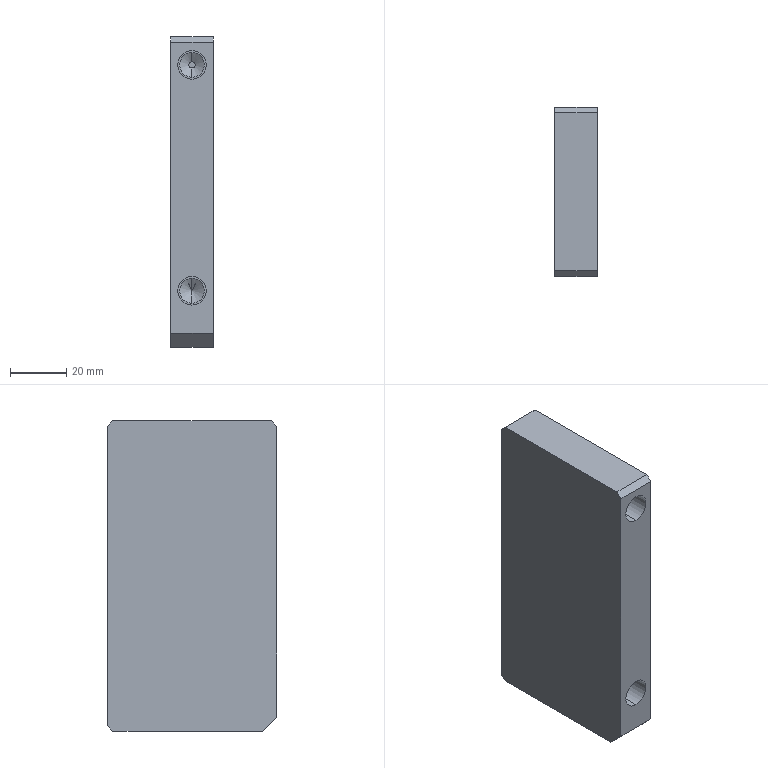Part | SolidWorks | features BaseBody 1 | 1 solid | 25 faces | box 15 x 60 x 110 mm | volume 93077 mm3 | plane 13 | cylinder 8 | cone 4 | commonest cylinder face diameters 8.8 x4 10.1 x4
STEP:
#1=CARTESIAN_POINT('',(257.5,55.,208.171));
#2=VERTEX_POINT('',#1);
#3=CARTESIAN_POINT('',(257.5,55.,198.071));
#4=VERTEX_POINT('',#3);
#5=CARTESIAN_POINT('',(257.5,55.,203.121));
#6=DIRECTION('',(0.,-1.,0.));
#7=DIRECTION('',(0.,0.,-1.));
#8=AXIS2_PLACEMENT_3D('',#5,#6,#7);
#9=CIRCLE('',#8,5.05);
#10=EDGE_CURVE('',#2,#4,#9,.T.);
#11=ORIENTED_EDGE('',*,*,#10,.F.);
#12=CARTESIAN_POINT('',(257.5,47.,208.171));
#13=VERTEX_POINT('',#12);
#14=CARTESIAN_POINT('',(257.5,55.,208.171));
#15=DIRECTION('',(0.,-1.,0.));
#16=VECTOR('',#15,1000.);
#17=LINE('',#14,#16);
#18=EDGE_CURVE('',#2,#13,#17,.T.);
#19=ORIENTED_EDGE('',*,*,#18,.T.);
#20=CARTESIAN_POINT('',(257.5,47.,198.071));
#21=VERTEX_POINT('',#20);
#22=CARTESIAN_POINT('',(257.5,47.,203.121));
#23=DIRECTION('',(0.,-1.,0.));
#24=DIRECTION('',(0.,0.,-1.));
#25=AXIS2_PLACEMENT_3D('',#22,#23,#24);
#26=CIRCLE('',#25,5.05);
#27=EDGE_CURVE('',#13,#21,#26,.T.);
#28=ORIENTED_EDGE('',*,*,#27,.T.);
#29=CARTESIAN_POINT('',(257.5,55.,198.071));
#30=DIRECTION('',(0.,-1.,0.));
#31=VECTOR('',#30,1000.);
#32=LINE('',#29,#31);
#33=EDGE_CURVE('',#4,#21,#32,.T.);
#34=ORIENTED_EDGE('',*,*,#33,.F.);
#35=EDGE_LOOP('',(#11,#19,#28,#34));
#36=FACE_OUTER_BOUND('',#35,.T.);
#37=CARTESIAN_POINT('',(257.5,55.,203.121));
#38=DIRECTION('',(0.,-1.,0.));
#39=DIRECTION('',(0.,0.,-1.));
#40=AXIS2_PLACEMENT_3D('',#37,#38,#39);
#41=CYLINDRICAL_SURFACE('',#40,5.05);
#42=ADVANCED_FACE('',(#36),#41,.F.);
#43=CARTESIAN_POINT('',(257.5,55.,128.171));
#44=VERTEX_POINT('',#43);
#45=CARTESIAN_POINT('',(257.5,55.,118.071));
#46=VERTEX_POINT('',#45);
#47=CARTESIAN_POINT('',(257.5,55.,123.121));
#48=DIRECTION('',(0.,-1.,0.));
#49=DIRECTION('',(0.,0.,-1.));
#50=AXIS2_PLACEMENT_3D('',#47,#48,#49);
#51=CIRCLE('',#50,5.05);
#52=EDGE_CURVE('',#44,#46,#51,.T.);
#53=ORIENTED_EDGE('',*,*,#52,.F.);
#54=CARTESIAN_POINT('',(257.5,47.,128.171));
#55=VERTEX_POINT('',#54);
#56=CARTESIAN_POINT('',(257.5,55.,128.171));
#57=DIRECTION('',(0.,-1.,0.));
#58=VECTOR('',#57,1000.);
#59=LINE('',#56,#58);
#60=EDGE_CURVE('',#44,#55,#59,.T.);
#61=ORIENTED_EDGE('',*,*,#60,.T.);
#62=CARTESIAN_POINT('',(257.5,47.,118.071));
#63=VERTEX_POINT('',#62);
#64=CARTESIAN_POINT('',(257.5,47.,123.121));
#65=DIRECTION('',(0.,-1.,0.));
#66=DIRECTION('',(0.,0.,-1.));
#67=AXIS2_PLACEMENT_3D('',#64,#65,#66);
#68=CIRCLE('',#67,5.05);
#69=EDGE_CURVE('',#55,#63,#68,.T.);
#70=ORIENTED_EDGE('',*,*,#69,.T.);
#71=CARTESIAN_POINT('',(257.5,55.,118.071));
#72=DIRECTION('',(0.,-1.,0.));
#73=VECTOR('',#72,1000.);
#74=LINE('',#71,#73);
#75=EDGE_CURVE('',#46,#63,#74,.T.);
#76=ORIENTED_EDGE('',*,*,#75,.F.);
#77=EDGE_LOOP('',(#53,#61,#70,#76));
#78=FACE_OUTER_BOUND('',#77,.T.);
#79=CARTESIAN_POINT('',(257.5,55.,123.121));
#80=DIRECTION('',(0.,-1.,0.));
#81=DIRECTION('',(0.,0.,-1.));
#82=AXIS2_PLACEMENT_3D('',#79,#80,#81);
#83=CYLINDRICAL_SURFACE('',#82,5.05);
#84=ADVANCED_FACE('',(#78),#83,.F.);
#85=CARTESIAN_POINT('',(257.5,90.,207.521));
#86=VERTEX_POINT('',#85);
#87=CARTESIAN_POINT('',(257.5,90.,198.721));
#88=VERTEX_POINT('',#87);
#89=CARTESIAN_POINT('',(257.5,90.,203.121));
#90=DIRECTION('',(0.,-1.,0.));
#91=DIRECTION('',(0.,0.,-1.));
#92=AXIS2_PLACEMENT_3D('',#89,#90,#91);
#93=CIRCLE('',#92,4.4);
#94=EDGE_CURVE('',#86,#88,#93,.T.);
#95=ORIENTED_EDGE('',*,*,#94,.F.);
#96=CARTESIAN_POINT('',(257.5,55.,207.521));
#97=VERTEX_POINT('',#96);
#98=CARTESIAN_POINT('',(257.5,55.,207.521));
#99=DIRECTION('',(0.,-1.,0.));
#100=VECTOR('',#99,1000.);
#101=LINE('',#98,#100);
#102=EDGE_CURVE('',#86,#97,#101,.T.);
#103=ORIENTED_EDGE('',*,*,#102,.T.);
#104=CARTESIAN_POINT('',(257.5,55.,198.721));
#105=VERTEX_POINT('',#104);
#106=CARTESIAN_POINT('',(257.5,55.,203.121));
#107=DIRECTION('',(0.,1.,0.));
#108=DIRECTION('',(0.,0.,-1.));
#109=AXIS2_PLACEMENT_3D('',#106,#107,#108);
#110=CIRCLE('',#109,4.4);
#111=EDGE_CURVE('',#105,#97,#110,.T.);
#112=ORIENTED_EDGE('',*,*,#111,.F.);
#113=CARTESIAN_POINT('',(257.5,55.,198.721));
#114=DIRECTION('',(0.,-1.,0.));
#115=VECTOR('',#114,1000.);
#116=LINE('',#113,#115);
#117=EDGE_CURVE('',#88,#105,#116,.T.);
#118=ORIENTED_EDGE('',*,*,#117,.F.);
#119=EDGE_LOOP('',(#95,#103,#112,#118));
#120=FACE_OUTER_BOUND('',#119,.T.);
#121=CARTESIAN_POINT('',(257.5,55.,203.121));
#122=DIRECTION('',(0.,-1.,0.));
#123=DIRECTION('',(0.,0.,-1.));
#124=AXIS2_PLACEMENT_3D('',#121,#122,#123);
#125=CYLINDRICAL_SURFACE('',#124,4.4);
#126=ADVANCED_FACE('',(#120),#125,.F.);
#127=CARTESIAN_POINT('',(257.5,90.,127.521));
#128=VERTEX_POINT('',#127);
#129=CARTESIAN_POINT('',(257.5,90.,118.721));
#130=VERTEX_POINT('',#129);
#131=CARTESIAN_POINT('',(257.5,90.,123.121));
#132=DIRECTION('',(0.,-1.,0.));
#133=DIRECTION('',(0.,0.,-1.));
#134=AXIS2_PLACEMENT_3D('',#131,#132,#133);
#135=CIRCLE('',#134,4.4);
#136=EDGE_CURVE('',#128,#130,#135,.T.);
#137=ORIENTED_EDGE('',*,*,#136,.F.);
#138=CARTESIAN_POINT('',(257.5,55.,127.521));
#139=VERTEX_POINT('',#138);
#140=CARTESIAN_POINT('',(257.5,55.,127.521));
#141=DIRECTION('',(0.,-1.,0.));
#142=VECTOR('',#141,1000.);
#143=LINE('',#140,#142);
#144=EDGE_CURVE('',#128,#139,#143,.T.);
#145=ORIENTED_EDGE('',*,*,#144,.T.);
#146=CARTESIAN_POINT('',(257.5,55.,118.721));
#147=VERTEX_POINT('',#146);
#148=CARTESIAN_POINT('',(257.5,55.,123.121));
#149=DIRECTION('',(0.,1.,0.));
#150=DIRECTION('',(0.,0.,-1.));
#151=AXIS2_PLACEMENT_3D('',#148,#149,#150);
#152=CIRCLE('',#151,4.4);
#153=EDGE_CURVE('',#147,#139,#152,.T.);
#154=ORIENTED_EDGE('',*,*,#153,.F.);
#155=CARTESIAN_POINT('',(257.5,55.,118.721));
#156=DIRECTION('',(0.,-1.,0.));
#157=VECTOR('',#156,1000.);
#158=LINE('',#155,#157);
#159=EDGE_CURVE('',#130,#147,#158,.T.);
#160=ORIENTED_EDGE('',*,*,#159,.F.);
#161=EDGE_LOOP('',(#137,#145,#154,#160));
#162=FACE_OUTER_BOUND('',#161,.T.);
#163=CARTESIAN_POINT('',(257.5,55.,123.121));
#164=DIRECTION('',(0.,-1.,0.));
#165=DIRECTION('',(0.,0.,-1.));
#166=AXIS2_PLACEMENT_3D('',#163,#164,#165);
#167=CYLINDRICAL_SURFACE('',#166,4.4);
#168=ADVANCED_FACE('',(#162),#167,.F.);
#169=CARTESIAN_POINT('',(257.5,92.,204.193));
#170=VERTEX_POINT('',#169);
#171=CARTESIAN_POINT('',(257.5,92.,202.05));
#172=VERTEX_POINT('',#171);
#173=CARTESIAN_POINT('',(257.5,92.,203.121));
#174=DIRECTION('',(0.,-1.,0.));
#175=DIRECTION('',(0.,0.,-1.));
#176=AXIS2_PLACEMENT_3D('',#173,#174,#175);
#177=CIRCLE('',#176,1.071);
#178=EDGE_CURVE('',#170,#172,#177,.T.);
#179=ORIENTED_EDGE('',*,*,#178,.F.);
#180=CARTESIAN_POINT('',(257.5,90.,207.521));
#181=DIRECTION('',(0.,-0.515,0.8572));
#182=VECTOR('',#181,1000.);
#183=LINE('',#180,#182);
#184=EDGE_CURVE('',#170,#86,#183,.T.);
#185=ORIENTED_EDGE('',*,*,#184,.T.);
#186=ORIENTED_EDGE('',*,*,#94,.T.);
#187=CARTESIAN_POINT('',(257.5,90.,198.721));
#188=DIRECTION('',(0.,-0.515,-0.8572));
#189=VECTOR('',#188,1000.);
#190=LINE('',#187,#189);
#191=EDGE_CURVE('',#172,#88,#190,.T.);
#192=ORIENTED_EDGE('',*,*,#191,.F.);
#193=EDGE_LOOP('',(#179,#185,#186,#192));
#194=FACE_OUTER_BOUND('',#193,.T.);
#195=CARTESIAN_POINT('',(257.5,90.,203.121));
#196=DIRECTION('',(0.,-1.,0.));
#197=DIRECTION('',(0.,0.,-1.));
#198=AXIS2_PLACEMENT_3D('',#195,#196,#197);
#199=CONICAL_SURFACE('',#198,4.4,1.03);
#200=ADVANCED_FACE('',(#194),#199,.F.);
#201=CARTESIAN_POINT('',(257.5,92.644,123.121));
#202=VERTEX_POINT('',#201);
#203=CARTESIAN_POINT('',(257.5,90.,118.721));
#204=DIRECTION('',(0.,-0.515,-0.8572));
#205=VECTOR('',#204,1000.);
#206=LINE('',#203,#205);
#207=EDGE_CURVE('',#202,#130,#206,.T.);
#208=ORIENTED_EDGE('',*,*,#207,.F.);
#209=CARTESIAN_POINT('',(257.5,90.,127.521));
#210=DIRECTION('',(0.,-0.515,0.8572));
#211=VECTOR('',#210,1000.);
#212=LINE('',#209,#211);
#213=EDGE_CURVE('',#202,#128,#212,.T.);
#214=ORIENTED_EDGE('',*,*,#213,.T.);
#215=ORIENTED_EDGE('',*,*,#136,.T.);
#216=EDGE_LOOP('',(#208,#214,#215));
#217=FACE_OUTER_BOUND('',#216,.T.);
#218=CARTESIAN_POINT('',(257.5,90.,123.121));
#219=DIRECTION('',(0.,-1.,0.));
#220=DIRECTION('',(0.,0.,-1.));
#221=AXIS2_PLACEMENT_3D('',#218,#219,#220);
#222=CONICAL_SURFACE('',#221,4.4,1.03);
#223=ADVANCED_FACE('',(#217),#222,.F.);
#224=CARTESIAN_POINT('',(250.,105.,103.121));
#225=VERTEX_POINT('',#224);
#226=CARTESIAN_POINT('',(250.,107.,105.121));
#227=VERTEX_POINT('',#226);
#228=CARTESIAN_POINT('',(250.,105.,103.121));
#229=DIRECTION('',(0.,0.7071,0.7071));
#230=VECTOR('',#229,1000.);
#231=LINE('',#228,#230);
#232=EDGE_CURVE('',#225,#227,#231,.T.);
#233=ORIENTED_EDGE('',*,*,#232,.F.);
#234=CARTESIAN_POINT('',(250.,52.,103.121));
#235=VERTEX_POINT('',#234);
#236=CARTESIAN_POINT('',(250.,47.,103.121));
#237=DIRECTION('',(0.,1.,0.));
#238=VECTOR('',#237,1000.);
#239=LINE('',#236,#238);
#240=EDGE_CURVE('',#235,#225,#239,.T.);
#241=ORIENTED_EDGE('',*,*,#240,.F.);
#242=CARTESIAN_POINT('',(250.,47.,108.121));
#243=VERTEX_POINT('',#242);
#244=CARTESIAN_POINT('',(250.,47.,108.121));
#245=DIRECTION('',(0.,0.7071,-0.7071));
#246=VECTOR('',#245,1000.);
#247=LINE('',#244,#246);
#248=EDGE_CURVE('',#243,#235,#247,.T.);
#249=ORIENTED_EDGE('',*,*,#248,.F.);
#250=CARTESIAN_POINT('',(250.,47.,211.121));
#251=VERTEX_POINT('',#250);
#252=CARTESIAN_POINT('',(250.,47.,103.121));
#253=DIRECTION('',(0.,0.,-1.));
#254=VECTOR('',#253,1000.);
#255=LINE('',#252,#254);
#256=EDGE_CURVE('',#251,#243,#255,.T.);
#257=ORIENTED_EDGE('',*,*,#256,.F.);
#258=CARTESIAN_POINT('',(250.,49.,213.121));
#259=VERTEX_POINT('',#258);
#260=CARTESIAN_POINT('',(250.,49.,213.121));
#261=DIRECTION('',(0.,-0.7071,-0.7071));
#262=VECTOR('',#261,1000.);
#263=LINE('',#260,#262);
#264=EDGE_CURVE('',#259,#251,#263,.T.);
#265=ORIENTED_EDGE('',*,*,#264,.F.);
#266=CARTESIAN_POINT('',(250.,105.,213.121));
#267=VERTEX_POINT('',#266);
#268=CARTESIAN_POINT('',(250.,47.,213.121));
#269=DIRECTION('',(0.,-1.,0.));
#270=VECTOR('',#269,1000.);
#271=LINE('',#268,#270);
#272=EDGE_CURVE('',#267,#259,#271,.T.);
#273=ORIENTED_EDGE('',*,*,#272,.F.);
#274=CARTESIAN_POINT('',(250.,107.,211.121));
#275=VERTEX_POINT('',#274);
#276=CARTESIAN_POINT('',(250.,107.,211.121));
#277=DIRECTION('',(0.,-0.7071,0.7071));
#278=VECTOR('',#277,1000.);
#279=LINE('',#276,#278);
#280=EDGE_CURVE('',#275,#267,#279,.T.);
#281=ORIENTED_EDGE('',*,*,#280,.F.);
#282=CARTESIAN_POINT('',(250.,107.,103.121));
#283=DIRECTION('',(0.,0.,1.));
#284=VECTOR('',#283,1000.);
#285=LINE('',#282,#284);
#286=EDGE_CURVE('',#227,#275,#285,.T.);
#287=ORIENTED_EDGE('',*,*,#286,.F.);
#288=EDGE_LOOP('',(#233,#241,#249,#257,#265,#273,#281,#287));
#289=FACE_OUTER_BOUND('',#288,.T.);
#290=CARTESIAN_POINT('',(250.,47.,103.121));
#291=DIRECTION('',(1.,0.,0.));
#292=DIRECTION('',(0.,0.,-1.));
#293=AXIS2_PLACEMENT_3D('',#290,#291,#292);
#294=PLANE('',#293);
#295=ADVANCED_FACE('',(#289),#294,.F.);
#296=CARTESIAN_POINT('',(265.,107.,105.121));
#297=VERTEX_POINT('',#296);
#298=CARTESIAN_POINT('',(177.5,107.,105.121));
#299=DIRECTION('',(1.,0.,0.));
#300=VECTOR('',#299,1000.);
#301=LINE('',#298,#300);
#302=EDGE_CURVE('',#227,#297,#301,.T.);
#303=ORIENTED_EDGE('',*,*,#302,.F.);
#304=ORIENTED_EDGE('',*,*,#286,.T.);
#305=CARTESIAN_POINT('',(265.,107.,211.121));
#306=VERTEX_POINT('',#305);
#307=CARTESIAN_POINT('',(177.5,107.,211.121));
#308=DIRECTION('',(-1.,0.,0.));
#309=VECTOR('',#308,1000.);
#310=LINE('',#307,#309);
#311=EDGE_CURVE('',#306,#275,#310,.T.);
#312=ORIENTED_EDGE('',*,*,#311,.F.);
#313=CARTESIAN_POINT('',(265.,107.,153.121));
#314=DIRECTION('',(0.,0.,1.));
#315=VECTOR('',#314,1000.);
#316=LINE('',#313,#315);
#317=EDGE_CURVE('',#297,#306,#316,.T.);
#318=ORIENTED_EDGE('',*,*,#317,.F.);
#319=EDGE_LOOP('',(#303,#304,#312,#318));
#320=FACE_OUTER_BOUND('',#319,.T.);
#321=CARTESIAN_POINT('',(177.5,107.,153.121));
#322=DIRECTION('',(0.,-1.,0.));
#323=DIRECTION('',(0.,0.,-1.));
#324=AXIS2_PLACEMENT_3D('',#321,#322,#323);
#325=PLANE('',#324);
#326=ADVANCED_FACE('',(#320),#325,.F.);
#327=ORIENTED_EDGE('',*,*,#302,.T.);
#328=CARTESIAN_POINT('',(265.,105.,103.121));
#329=VERTEX_POINT('',#328);
#330=CARTESIAN_POINT('',(265.,105.,103.121));
#331=DIRECTION('',(0.,0.7071,0.7071));
#332=VECTOR('',#331,1000.);
#333=LINE('',#330,#332);
#334=EDGE_CURVE('',#329,#297,#333,.T.);
#335=ORIENTED_EDGE('',*,*,#334,.F.);
#336=CARTESIAN_POINT('',(90.,105.,103.121));
#337=DIRECTION('',(1.,0.,0.));
#338=VECTOR('',#337,1000.);
#339=LINE('',#336,#338);
#340=EDGE_CURVE('',#225,#329,#339,.T.);
#341=ORIENTED_EDGE('',*,*,#340,.F.);
#342=ORIENTED_EDGE('',*,*,#232,.T.);
#343=EDGE_LOOP('',(#327,#335,#341,#342));
#344=FACE_OUTER_BOUND('',#343,.T.);
#345=CARTESIAN_POINT('',(90.,105.,103.121));
#346=DIRECTION('',(0.,-0.7071,0.7071));
#347=DIRECTION('',(0.,-0.7071,-0.7071));
#348=AXIS2_PLACEMENT_3D('',#345,#346,#347);
#349=PLANE('',#348);
#350=ADVANCED_FACE('',(#344),#349,.F.);
#351=ORIENTED_EDGE('',*,*,#340,.T.);
#352=CARTESIAN_POINT('',(265.,52.,103.121));
#353=VERTEX_POINT('',#352);
#354=CARTESIAN_POINT('',(265.,92.,103.121));
#355=DIRECTION('',(0.,1.,0.));
#356=VECTOR('',#355,1000.);
#357=LINE('',#354,#356);
#358=EDGE_CURVE('',#353,#329,#357,.T.);
#359=ORIENTED_EDGE('',*,*,#358,.F.);
#360=CARTESIAN_POINT('',(90.,52.,103.121));
#361=DIRECTION('',(1.,0.,0.));
#362=VECTOR('',#361,1000.);
#363=LINE('',#360,#362);
#364=EDGE_CURVE('',#235,#353,#363,.T.);
#365=ORIENTED_EDGE('',*,*,#364,.F.);
#366=ORIENTED_EDGE('',*,*,#240,.T.);
#367=EDGE_LOOP('',(#351,#359,#365,#366));
#368=FACE_OUTER_BOUND('',#367,.T.);
#369=CARTESIAN_POINT('',(90.,92.,103.121));
#370=DIRECTION('',(0.,0.,1.));
#371=DIRECTION('',(1.,0.,0.));
#372=AXIS2_PLACEMENT_3D('',#369,#370,#371);
#373=PLANE('',#372);
#374=ADVANCED_FACE('',(#368),#373,.F.);
#375=ORIENTED_EDGE('',*,*,#364,.T.);
#376=CARTESIAN_POINT('',(265.,47.,108.121));
#377=VERTEX_POINT('',#376);
#378=CARTESIAN_POINT('',(265.,47.,108.121));
#379=DIRECTION('',(0.,0.7071,-0.7071));
#380=VECTOR('',#379,1000.);
#381=LINE('',#378,#380);
#382=EDGE_CURVE('',#377,#353,#381,.T.);
#383=ORIENTED_EDGE('',*,*,#382,.F.);
#384=CARTESIAN_POINT('',(177.5,47.,108.121));
#385=DIRECTION('',(1.,0.,0.));
#386=VECTOR('',#385,1000.);
#387=LINE('',#384,#386);
#388=EDGE_CURVE('',#243,#377,#387,.T.);
#389=ORIENTED_EDGE('',*,*,#388,.F.);
#390=ORIENTED_EDGE('',*,*,#248,.T.);
#391=EDGE_LOOP('',(#375,#383,#389,#390));
#392=FACE_OUTER_BOUND('',#391,.T.);
#393=CARTESIAN_POINT('',(177.5,47.,108.121));
#394=DIRECTION('',(0.,0.7071,0.7071));
#395=DIRECTION('',(0.,-0.7071,0.7071));
#396=AXIS2_PLACEMENT_3D('',#393,#394,#395);
#397=PLANE('',#396);
#398=ADVANCED_FACE('',(#392),#397,.F.);
#399=CARTESIAN_POINT('',(265.,47.,211.121));
#400=VERTEX_POINT('',#399);
#401=CARTESIAN_POINT('',(177.5,47.,211.121));
#402=DIRECTION('',(1.,0.,0.));
#403=VECTOR('',#402,1000.);
#404=LINE('',#401,#403);
#405=EDGE_CURVE('',#251,#400,#404,.T.);
#406=ORIENTED_EDGE('',*,*,#405,.F.);
#407=ORIENTED_EDGE('',*,*,#256,.T.);
#408=ORIENTED_EDGE('',*,*,#388,.T.);
#409=CARTESIAN_POINT('',(265.,47.,153.121));
#410=DIRECTION('',(0.,0.,-1.));
#411=VECTOR('',#410,1000.);
#412=LINE('',#409,#411);
#413=EDGE_CURVE('',#400,#377,#412,.T.);
#414=ORIENTED_EDGE('',*,*,#413,.F.);
#415=EDGE_LOOP('',(#406,#407,#408,#414));
#416=FACE_OUTER_BOUND('',#415,.T.);
#417=CARTESIAN_POINT('',(257.5,47.,203.121));
#418=DIRECTION('',(0.,-1.,0.));
#419=DIRECTION('',(0.,0.,-1.));
#420=AXIS2_PLACEMENT_3D('',#417,#418,#419);
#421=CIRCLE('',#420,5.05);
#422=EDGE_CURVE('',#21,#13,#421,.T.);
#423=ORIENTED_EDGE('',*,*,#422,.F.);
#424=ORIENTED_EDGE('',*,*,#27,.F.);
#425=EDGE_LOOP('',(#423,#424));
#426=FACE_BOUND('',#425,.T.);
#427=CARTESIAN_POINT('',(257.5,47.,123.121));
#428=DIRECTION('',(0.,-1.,0.));
#429=DIRECTION('',(0.,0.,-1.));
#430=AXIS2_PLACEMENT_3D('',#427,#428,#429);
#431=CIRCLE('',#430,5.05);
#432=EDGE_CURVE('',#63,#55,#431,.T.);
#433=ORIENTED_EDGE('',*,*,#432,.F.);
#434=ORIENTED_EDGE('',*,*,#69,.F.);
#435=EDGE_LOOP('',(#433,#434));
#436=FACE_BOUND('',#435,.T.);
#437=CARTESIAN_POINT('',(177.5,47.,153.121));
#438=DIRECTION('',(0.,1.,0.));
#439=DIRECTION('',(0.,0.,1.));
#440=AXIS2_PLACEMENT_3D('',#437,#438,#439);
#441=PLANE('',#440);
#442=ADVANCED_FACE('',(#416,#426,#436),#441,.F.);
#443=CARTESIAN_POINT('',(265.,49.,213.121));
#444=VERTEX_POINT('',#443);
#445=CARTESIAN_POINT('',(265.,49.,213.121));
#446=DIRECTION('',(0.,0.7071,0.7071));
#447=VECTOR('',#446,1000.);
#448=LINE('',#445,#447);
#449=EDGE_CURVE('',#400,#444,#448,.T.);
#450=ORIENTED_EDGE('',*,*,#449,.T.);
#451=CARTESIAN_POINT('',(177.5,49.,213.121));
#452=DIRECTION('',(-1.,0.,0.));
#453=VECTOR('',#452,1000.);
#454=LINE('',#451,#453);
#455=EDGE_CURVE('',#444,#259,#454,.T.);
#456=ORIENTED_EDGE('',*,*,#455,.T.);
#457=ORIENTED_EDGE('',*,*,#264,.T.);
#458=ORIENTED_EDGE('',*,*,#405,.T.);
#459=EDGE_LOOP('',(#450,#456,#457,#458));
#460=FACE_OUTER_BOUND('',#459,.T.);
#461=CARTESIAN_POINT('',(177.5,49.,213.121));
#462=DIRECTION('',(0.,-0.7071,0.7071));
#463=DIRECTION('',(0.,-0.7071,-0.7071));
#464=AXIS2_PLACEMENT_3D('',#461,#462,#463);
#465=PLANE('',#464);
#466=ADVANCED_FACE('',(#460),#465,.T.);
#467=ORIENTED_EDGE('',*,*,#272,.T.);
#468=ORIENTED_EDGE('',*,*,#455,.F.);
#469=CARTESIAN_POINT('',(265.,105.,213.121));
#470=VERTEX_POINT('',#469);
#471=CARTESIAN_POINT('',(265.,107.,213.121));
#472=DIRECTION('',(0.,1.,0.));
#473=VECTOR('',#472,1000.);
#474=LINE('',#471,#473);
#475=EDGE_CURVE('',#444,#470,#474,.T.);
#476=ORIENTED_EDGE('',*,*,#475,.T.);
#477=CARTESIAN_POINT('',(177.5,105.,213.121));
#478=DIRECTION('',(-1.,0.,0.));
#479=VECTOR('',#478,1000.);
#480=LINE('',#477,#479);
#481=EDGE_CURVE('',#470,#267,#480,.T.);
#482=ORIENTED_EDGE('',*,*,#481,.T.);
#483=EDGE_LOOP('',(#467,#468,#476,#482));
#484=FACE_OUTER_BOUND('',#483,.T.);
#485=CARTESIAN_POINT('',(177.5,107.,213.121));
#486=DIRECTION('',(0.,0.,1.));
#487=DIRECTION('',(1.,0.,0.));
#488=AXIS2_PLACEMENT_3D('',#485,#486,#487);
#489=PLANE('',#488);
#490=ADVANCED_FACE('',(#484),#489,.T.);
#491=CARTESIAN_POINT('',(265.,107.,211.121));
#492=DIRECTION('',(0.,0.7071,-0.7071));
#493=VECTOR('',#492,1000.);
#494=LINE('',#491,#493);
#495=EDGE_CURVE('',#470,#306,#494,.T.);
#496=ORIENTED_EDGE('',*,*,#495,.T.);
#497=ORIENTED_EDGE('',*,*,#311,.T.);
#498=ORIENTED_EDGE('',*,*,#280,.T.);
#499=ORIENTED_EDGE('',*,*,#481,.F.);
#500=EDGE_LOOP('',(#496,#497,#498,#499));
#501=FACE_OUTER_BOUND('',#500,.T.);
#502=CARTESIAN_POINT('',(177.5,107.,211.121));
#503=DIRECTION('',(0.,0.7071,0.7071));
#504=DIRECTION('',(0.,-0.7071,0.7071));
#505=AXIS2_PLACEMENT_3D('',#502,#503,#504);
#506=PLANE('',#505);
#507=ADVANCED_FACE('',(#501),#506,.T.);
#508=ORIENTED_EDGE('',*,*,#334,.T.);
#509=ORIENTED_EDGE('',*,*,#317,.T.);
#510=ORIENTED_EDGE('',*,*,#495,.F.);
#511=ORIENTED_EDGE('',*,*,#475,.F.);
#512=ORIENTED_EDGE('',*,*,#449,.F.);
#513=ORIENTED_EDGE('',*,*,#413,.T.);
#514=ORIENTED_EDGE('',*,*,#382,.T.);
#515=ORIENTED_EDGE('',*,*,#358,.T.);
#516=EDGE_LOOP('',(#508,#509,#510,#511,#512,#513,#514,#515));
#517=FACE_OUTER_BOUND('',#516,.T.);
#518=CARTESIAN_POINT('',(265.,92.,103.121));
#519=DIRECTION('',(-1.,0.,0.));
#520=DIRECTION('',(0.,0.,1.));
#521=AXIS2_PLACEMENT_3D('',#518,#519,#520);
#522=PLANE('',#521);
#523=ADVANCED_FACE('',(#517),#522,.F.);
#524=ORIENTED_EDGE('',*,*,#18,.F.);
#525=CARTESIAN_POINT('',(257.5,55.,203.121));
#526=DIRECTION('',(0.,-1.,0.));
#527=DIRECTION('',(0.,0.,-1.));
#528=AXIS2_PLACEMENT_3D('',#525,#526,#527);
#529=CIRCLE('',#528,5.05);
#530=EDGE_CURVE('',#4,#2,#529,.T.);
#531=ORIENTED_EDGE('',*,*,#530,.F.);
#532=ORIENTED_EDGE('',*,*,#33,.T.);
#533=ORIENTED_EDGE('',*,*,#422,.T.);
#534=EDGE_LOOP('',(#524,#531,#532,#533));
#535=FACE_OUTER_BOUND('',#534,.T.);
#536=CARTESIAN_POINT('',(257.5,55.,203.121));
#537=DIRECTION('',(0.,-1.,0.));
#538=DIRECTION('',(0.,0.,-1.));
#539=AXIS2_PLACEMENT_3D('',#536,#537,#538);
#540=CYLINDRICAL_SURFACE('',#539,5.05);
#541=ADVANCED_FACE('',(#535),#540,.F.);
#542=ORIENTED_EDGE('',*,*,#60,.F.);
#543=CARTESIAN_POINT('',(257.5,55.,123.121));
#544=DIRECTION('',(0.,-1.,0.));
#545=DIRECTION('',(0.,0.,-1.));
#546=AXIS2_PLACEMENT_3D('',#543,#544,#545);
#547=CIRCLE('',#546,5.05);
#548=EDGE_CURVE('',#46,#44,#547,.T.);
#549=ORIENTED_EDGE('',*,*,#548,.F.);
#550=ORIENTED_EDGE('',*,*,#75,.T.);
#551=ORIENTED_EDGE('',*,*,#432,.T.);
#552=EDGE_LOOP('',(#542,#549,#550,#551));
#553=FACE_OUTER_BOUND('',#552,.T.);
#554=CARTESIAN_POINT('',(257.5,55.,123.121));
#555=DIRECTION('',(0.,-1.,0.));
#556=DIRECTION('',(0.,0.,-1.));
#557=AXIS2_PLACEMENT_3D('',#554,#555,#556);
#558=CYLINDRICAL_SURFACE('',#557,5.05);
#559=ADVANCED_FACE('',(#553),#558,.F.);
#560=ORIENTED_EDGE('',*,*,#530,.T.);
#561=ORIENTED_EDGE('',*,*,#10,.T.);
#562=EDGE_LOOP('',(#560,#561));
#563=FACE_OUTER_BOUND('',#562,.T.);
#564=ORIENTED_EDGE('',*,*,#111,.T.);
#565=CARTESIAN_POINT('',(257.5,55.,203.121));
#566=DIRECTION('',(0.,1.,0.));
#567=DIRECTION('',(0.,0.,-1.));
#568=AXIS2_PLACEMENT_3D('',#565,#566,#567);
#569=CIRCLE('',#568,4.4);
#570=EDGE_CURVE('',#97,#105,#569,.T.);
#571=ORIENTED_EDGE('',*,*,#570,.T.);
#572=EDGE_LOOP('',(#564,#571));
#573=FACE_BOUND('',#572,.T.);
#574=CARTESIAN_POINT('',(257.5,55.,203.121));
#575=DIRECTION('',(0.,-1.,0.));
#576=DIRECTION('',(0.,0.,-1.));
#577=AXIS2_PLACEMENT_3D('',#574,#575,#576);
#578=PLANE('',#577);
#579=ADVANCED_FACE('',(#563,#573),#578,.T.);
#580=ORIENTED_EDGE('',*,*,#548,.T.);
#581=ORIENTED_EDGE('',*,*,#52,.T.);
#582=EDGE_LOOP('',(#580,#581));
#583=FACE_OUTER_BOUND('',#582,.T.);
#584=ORIENTED_EDGE('',*,*,#153,.T.);
#585=CARTESIAN_POINT('',(257.5,55.,123.121));
#586=DIRECTION('',(0.,1.,0.));
#587=DIRECTION('',(0.,0.,-1.));
#588=AXIS2_PLACEMENT_3D('',#585,#586,#587);
#589=CIRCLE('',#588,4.4);
#590=EDGE_CURVE('',#139,#147,#589,.T.);
#591=ORIENTED_EDGE('',*,*,#590,.T.);
#592=EDGE_LOOP('',(#584,#591));
#593=FACE_BOUND('',#592,.T.);
#594=CARTESIAN_POINT('',(257.5,55.,123.121));
#595=DIRECTION('',(0.,-1.,0.));
#596=DIRECTION('',(0.,0.,-1.));
#597=AXIS2_PLACEMENT_3D('',#594,#595,#596);
#598=PLANE('',#597);
#599=ADVANCED_FACE('',(#583,#593),#598,.T.);
#600=ORIENTED_EDGE('',*,*,#102,.F.);
#601=CARTESIAN_POINT('',(257.5,90.,203.121));
#602=DIRECTION('',(0.,-1.,0.));
#603=DIRECTION('',(0.,0.,-1.));
#604=AXIS2_PLACEMENT_3D('',#601,#602,#603);
#605=CIRCLE('',#604,4.4);
#606=EDGE_CURVE('',#88,#86,#605,.T.);
#607=ORIENTED_EDGE('',*,*,#606,.F.);
#608=ORIENTED_EDGE('',*,*,#117,.T.);
#609=ORIENTED_EDGE('',*,*,#570,.F.);
#610=EDGE_LOOP('',(#600,#607,#608,#609));
#611=FACE_OUTER_BOUND('',#610,.T.);
#612=CARTESIAN_POINT('',(257.5,55.,203.121));
#613=DIRECTION('',(0.,-1.,0.));
#614=DIRECTION('',(0.,0.,-1.));
#615=AXIS2_PLACEMENT_3D('',#612,#613,#614);
#616=CYLINDRICAL_SURFACE('',#615,4.4);
#617=ADVANCED_FACE('',(#611),#616,.F.);
#618=ORIENTED_EDGE('',*,*,#144,.F.);
#619=CARTESIAN_POINT('',(257.5,90.,123.121));
#620=DIRECTION('',(0.,-1.,0.));
#621=DIRECTION('',(0.,0.,-1.));
#622=AXIS2_PLACEMENT_3D('',#619,#620,#621);
#623=CIRCLE('',#622,4.4);
#624=EDGE_CURVE('',#130,#128,#623,.T.);
#625=ORIENTED_EDGE('',*,*,#624,.F.);
#626=ORIENTED_EDGE('',*,*,#159,.T.);
#627=ORIENTED_EDGE('',*,*,#590,.F.);
#628=EDGE_LOOP('',(#618,#625,#626,#627));
#629=FACE_OUTER_BOUND('',#628,.T.);
#630=CARTESIAN_POINT('',(257.5,55.,123.121));
#631=DIRECTION('',(0.,-1.,0.));
#632=DIRECTION('',(0.,0.,-1.));
#633=AXIS2_PLACEMENT_3D('',#630,#631,#632);
#634=CYLINDRICAL_SURFACE('',#633,4.4);
#635=ADVANCED_FACE('',(#629),#634,.F.);
#636=ORIENTED_EDGE('',*,*,#184,.F.);
#637=CARTESIAN_POINT('',(257.5,92.,203.121));
#638=DIRECTION('',(0.,-1.,0.));
#639=DIRECTION('',(0.,0.,-1.));
#640=AXIS2_PLACEMENT_3D('',#637,#638,#639);
#641=CIRCLE('',#640,1.071);
#642=EDGE_CURVE('',#172,#170,#641,.T.);
#643=ORIENTED_EDGE('',*,*,#642,.F.);
#644=ORIENTED_EDGE('',*,*,#191,.T.);
#645=ORIENTED_EDGE('',*,*,#606,.T.);
#646=EDGE_LOOP('',(#636,#643,#644,#645));
#647=FACE_OUTER_BOUND('',#646,.T.);
#648=CARTESIAN_POINT('',(257.5,90.,203.121));
#649=DIRECTION('',(0.,-1.,0.));
#650=DIRECTION('',(0.,0.,-1.));
#651=AXIS2_PLACEMENT_3D('',#648,#649,#650);
#652=CONICAL_SURFACE('',#651,4.4,1.03);
#653=ADVANCED_FACE('',(#647),#652,.F.);
#654=ORIENTED_EDGE('',*,*,#213,.F.);
#655=ORIENTED_EDGE('',*,*,#207,.T.);
#656=ORIENTED_EDGE('',*,*,#624,.T.);
#657=EDGE_LOOP('',(#654,#655,#656));
#658=FACE_OUTER_BOUND('',#657,.T.);
#659=CARTESIAN_POINT('',(257.5,90.,123.121));
#660=DIRECTION('',(0.,-1.,0.));
#661=DIRECTION('',(0.,0.,-1.));
#662=AXIS2_PLACEMENT_3D('',#659,#660,#661);
#663=CONICAL_SURFACE('',#662,4.4,1.03);
#664=ADVANCED_FACE('',(#658),#663,.F.);
#665=ORIENTED_EDGE('',*,*,#642,.T.);
#666=ORIENTED_EDGE('',*,*,#178,.T.);
#667=EDGE_LOOP('',(#665,#666));
#668=FACE_OUTER_BOUND('',#667,.T.);
#669=CARTESIAN_POINT('',(119.137,92.,153.121));
#670=DIRECTION('',(0.,-1.,0.));
#671=DIRECTION('',(0.,0.,-1.));
#672=AXIS2_PLACEMENT_3D('',#669,#670,#671);
#673=PLANE('',#672);
#674=ADVANCED_FACE('',(#668),#673,.T.);
#675=CLOSED_SHELL('',(#42,#84,#126,#168,#200,#223,#295,#326,#350,#374,#398,#442,#466,#490,#507,#523,#541,#559,#579,#599,#617,#635,#653,#664,#674));
#676=MANIFOLD_SOLID_BREP('',#675);
#677=CARTESIAN_POINT('',(0.,0.,0.));
#678=DIRECTION('',(0.,0.,1.));
#679=DIRECTION('',(1.,0.,0.));
#680=AXIS2_PLACEMENT_3D('',#677,#678,#679);
#681=(LENGTH_UNIT()NAMED_UNIT(*)SI_UNIT(.MILLI.,.METRE.));
#682=UNCERTAINTY_MEASURE_WITH_UNIT(LENGTH_MEASURE(0.00001),#681,'','');
#683=(NAMED_UNIT(*)PLANE_ANGLE_UNIT()SI_UNIT($,.RADIAN.));
#684=(NAMED_UNIT(*)SI_UNIT($,.STERADIAN.)SOLID_ANGLE_UNIT());
#685=(GEOMETRIC_REPRESENTATION_CONTEXT(3)GLOBAL_UNCERTAINTY_ASSIGNED_CONTEXT((#682))GLOBAL_UNIT_ASSIGNED_CONTEXT((#681,#683,#684))REPRESENTATION_CONTEXT('',''));
#686=ADVANCED_BREP_SHAPE_REPRESENTATION('',(#676,#680),#685);